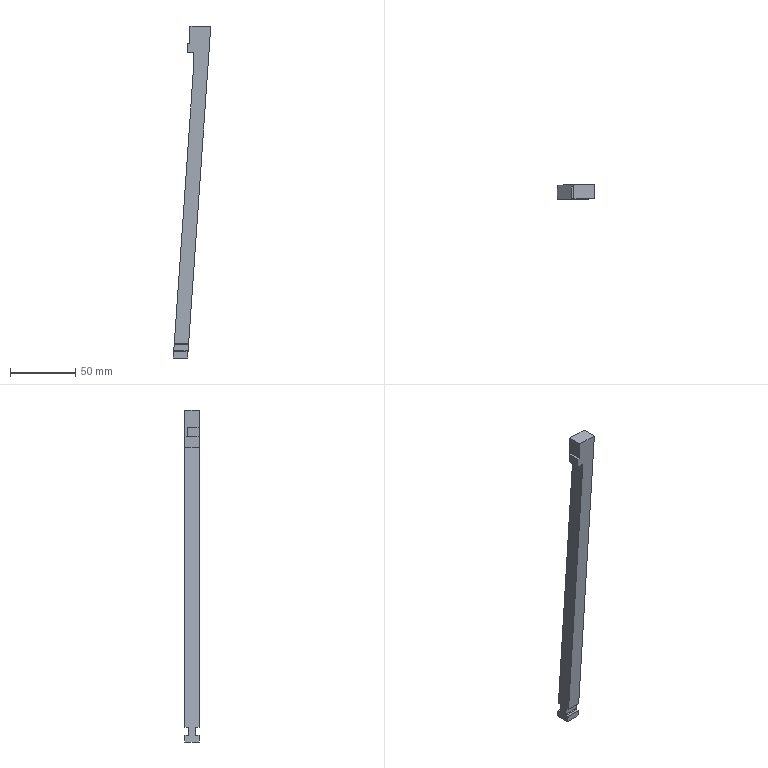Part | Creo | 1 solid | 100 faces | box 28.828 x 11 x 255.177 mm | volume 31691 mm3 | other 53 | plane 41 | cylinder 6 | commonest cylinder face diameters 1 x4 2.036 x1 32.111 x1